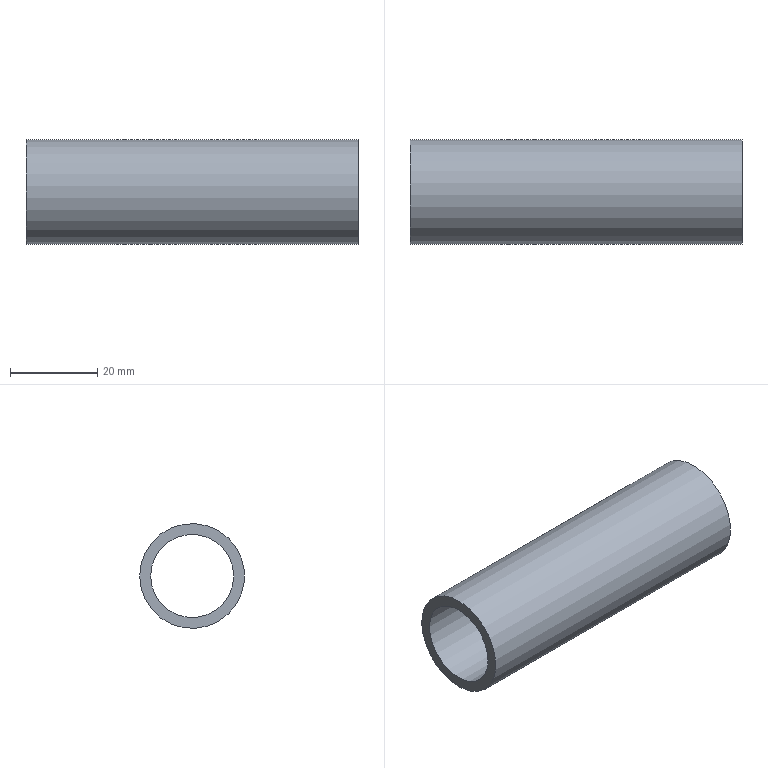Part | STEP file | 1-46.2 | 1 solid | 4 faces | box 76 x 24 x 24 mm | volume 12833 mm3 | plane 2 | cylinder 2 | commonest cylinder face diameters 19 x1 24 x1
STEP:
#1=CARTESIAN_POINT('',(0.,0.,0.));
#2=DIRECTION('',(0.,0.,1.));
#3=DIRECTION('',(1.,0.,0.));
#4=AXIS2_PLACEMENT_3D('',#1,#2,#3);
#5=CARTESIAN_POINT('',(38.,12.,0.));
#6=VERTEX_POINT('',#5);
#7=CARTESIAN_POINT('',(38.,0.,0.));
#8=DIRECTION('',(1.,0.,0.));
#9=DIRECTION('',(0.,1.,0.));
#10=AXIS2_PLACEMENT_3D('',#7,#8,#9);
#11=CIRCLE('',#10,12.);
#12=CARTESIAN_POINT('',(38.,-3.215,0.));
#13=DIRECTION('',(1.,0.,0.));
#14=DIRECTION('',(0.,1.,0.));
#15=AXIS2_PLACEMENT_3D('',#12,#13,#14);
#16=PLANE('',#15);
#17=CARTESIAN_POINT('',(3.215,0.));
#18=DIRECTION('',(1.,0.));
#19=AXIS2_PLACEMENT_2D('',#17,#18);
#20=CIRCLE('',#19,12.);
#21=(GEOMETRIC_REPRESENTATION_CONTEXT(2)PARAMETRIC_REPRESENTATION_CONTEXT()REPRESENTATION_CONTEXT('',''));
#22=DEFINITIONAL_REPRESENTATION('',(#20),#21);
#23=PCURVE('',#16,#22);
#24=CARTESIAN_POINT('',(38.,0.,0.));
#25=DIRECTION('',(-1.,0.,0.));
#26=DIRECTION('',(0.,1.,0.));
#27=AXIS2_PLACEMENT_3D('',#24,#25,#26);
#28=CYLINDRICAL_SURFACE('',#27,12.);
#29=CARTESIAN_POINT('',(6.283,0.));
#30=DIRECTION('',(-1.,0.));
#31=VECTOR('',#30,1.);
#32=LINE('',#29,#31);
#33=(GEOMETRIC_REPRESENTATION_CONTEXT(2)PARAMETRIC_REPRESENTATION_CONTEXT()REPRESENTATION_CONTEXT('',''));
#34=DEFINITIONAL_REPRESENTATION('',(#32),#33);
#35=PCURVE('',#28,#34);
#36=SURFACE_CURVE('',#11,(#23,#35),.PCURVE_S1.);
#37=EDGE_CURVE('',#6,#6,#36,.T.);
#38=ORIENTED_EDGE('',*,*,#37,.T.);
#39=EDGE_LOOP('',(#38));
#40=FACE_BOUND('',#39,.T.);
#41=CARTESIAN_POINT('',(38.,9.5,0.));
#42=VERTEX_POINT('',#41);
#43=CARTESIAN_POINT('',(38.,0.,0.));
#44=DIRECTION('',(-1.,0.,0.));
#45=DIRECTION('',(0.,1.,0.));
#46=AXIS2_PLACEMENT_3D('',#43,#44,#45);
#47=CIRCLE('',#46,9.5);
#48=CARTESIAN_POINT('',(12.715,0.));
#49=CARTESIAN_POINT('',(12.715,-16.454));
#50=CARTESIAN_POINT('',(-1.535,-8.227));
#51=CARTESIAN_POINT('',(-15.785,0.));
#52=CARTESIAN_POINT('',(-1.535,8.227));
#53=CARTESIAN_POINT('',(12.715,16.454));
#54=CARTESIAN_POINT('',(12.715,0.));
#55=(BOUNDED_CURVE()B_SPLINE_CURVE(2,(#48,#49,#50,#51,#52,#53,#54),.UNSPECIFIED.,.T.,.F.)B_SPLINE_CURVE_WITH_KNOTS((1,2,2,2,2,1),(-2.094,0.,2.094,4.189,6.283,8.378),.UNSPECIFIED.)CURVE()GEOMETRIC_REPRESENTATION_ITEM()RATIONAL_B_SPLINE_CURVE((1.,0.5,1.,0.5,1.,0.5,1.))REPRESENTATION_ITEM(''));
#56=(GEOMETRIC_REPRESENTATION_CONTEXT(2)PARAMETRIC_REPRESENTATION_CONTEXT()REPRESENTATION_CONTEXT('',''));
#57=DEFINITIONAL_REPRESENTATION('',(#55),#56);
#58=PCURVE('',#16,#57);
#59=CARTESIAN_POINT('',(38.,0.,0.));
#60=DIRECTION('',(-1.,0.,0.));
#61=DIRECTION('',(0.,1.,0.));
#62=AXIS2_PLACEMENT_3D('',#59,#60,#61);
#63=CYLINDRICAL_SURFACE('',#62,9.5);
#64=CARTESIAN_POINT('',(0.,0.));
#65=DIRECTION('',(1.,0.));
#66=VECTOR('',#65,1.);
#67=LINE('',#64,#66);
#68=(GEOMETRIC_REPRESENTATION_CONTEXT(2)PARAMETRIC_REPRESENTATION_CONTEXT()REPRESENTATION_CONTEXT('',''));
#69=DEFINITIONAL_REPRESENTATION('',(#67),#68);
#70=PCURVE('',#63,#69);
#71=SURFACE_CURVE('',#47,(#58,#70),.PCURVE_S1.);
#72=EDGE_CURVE('',#42,#42,#71,.T.);
#73=ORIENTED_EDGE('',*,*,#72,.T.);
#74=EDGE_LOOP('',(#73));
#75=FACE_BOUND('',#74,.T.);
#76=ADVANCED_FACE('',(#40,#75),#16,.T.);
#77=CARTESIAN_POINT('',(-38.,12.,0.));
#78=VERTEX_POINT('',#77);
#79=CARTESIAN_POINT('',(-38.,0.,0.));
#80=DIRECTION('',(1.,0.,0.));
#81=DIRECTION('',(0.,1.,0.));
#82=AXIS2_PLACEMENT_3D('',#79,#80,#81);
#83=CIRCLE('',#82,12.);
#84=CARTESIAN_POINT('',(-38.,-3.215,0.));
#85=DIRECTION('',(1.,0.,0.));
#86=DIRECTION('',(0.,1.,0.));
#87=AXIS2_PLACEMENT_3D('',#84,#85,#86);
#88=PLANE('',#87);
#89=CARTESIAN_POINT('',(3.215,0.));
#90=DIRECTION('',(1.,0.));
#91=AXIS2_PLACEMENT_2D('',#89,#90);
#92=CIRCLE('',#91,12.);
#93=(GEOMETRIC_REPRESENTATION_CONTEXT(2)PARAMETRIC_REPRESENTATION_CONTEXT()REPRESENTATION_CONTEXT('',''));
#94=DEFINITIONAL_REPRESENTATION('',(#92),#93);
#95=PCURVE('',#88,#94);
#96=CARTESIAN_POINT('',(6.283,76.));
#97=DIRECTION('',(-1.,0.));
#98=VECTOR('',#97,1.);
#99=LINE('',#96,#98);
#100=(GEOMETRIC_REPRESENTATION_CONTEXT(2)PARAMETRIC_REPRESENTATION_CONTEXT()REPRESENTATION_CONTEXT('',''));
#101=DEFINITIONAL_REPRESENTATION('',(#99),#100);
#102=PCURVE('',#28,#101);
#103=SURFACE_CURVE('',#83,(#95,#102),.PCURVE_S1.);
#104=EDGE_CURVE('',#78,#78,#103,.T.);
#105=ORIENTED_EDGE('',*,*,#104,.T.);
#106=EDGE_LOOP('',(#105));
#107=FACE_BOUND('',#106,.F.);
#108=CARTESIAN_POINT('',(-38.,9.5,0.));
#109=VERTEX_POINT('',#108);
#110=CARTESIAN_POINT('',(-38.,0.,0.));
#111=DIRECTION('',(-1.,0.,0.));
#112=DIRECTION('',(0.,1.,0.));
#113=AXIS2_PLACEMENT_3D('',#110,#111,#112);
#114=CIRCLE('',#113,9.5);
#115=CARTESIAN_POINT('',(12.715,0.));
#116=CARTESIAN_POINT('',(12.715,-16.454));
#117=CARTESIAN_POINT('',(-1.535,-8.227));
#118=CARTESIAN_POINT('',(-15.785,0.));
#119=CARTESIAN_POINT('',(-1.535,8.227));
#120=CARTESIAN_POINT('',(12.715,16.454));
#121=CARTESIAN_POINT('',(12.715,0.));
#122=(BOUNDED_CURVE()B_SPLINE_CURVE(2,(#115,#116,#117,#118,#119,#120,#121),.UNSPECIFIED.,.T.,.F.)B_SPLINE_CURVE_WITH_KNOTS((1,2,2,2,2,1),(-2.094,0.,2.094,4.189,6.283,8.378),.UNSPECIFIED.)CURVE()GEOMETRIC_REPRESENTATION_ITEM()RATIONAL_B_SPLINE_CURVE((1.,0.5,1.,0.5,1.,0.5,1.))REPRESENTATION_ITEM(''));
#123=(GEOMETRIC_REPRESENTATION_CONTEXT(2)PARAMETRIC_REPRESENTATION_CONTEXT()REPRESENTATION_CONTEXT('',''));
#124=DEFINITIONAL_REPRESENTATION('',(#122),#123);
#125=PCURVE('',#88,#124);
#126=CARTESIAN_POINT('',(0.,76.));
#127=DIRECTION('',(1.,0.));
#128=VECTOR('',#127,1.);
#129=LINE('',#126,#128);
#130=(GEOMETRIC_REPRESENTATION_CONTEXT(2)PARAMETRIC_REPRESENTATION_CONTEXT()REPRESENTATION_CONTEXT('',''));
#131=DEFINITIONAL_REPRESENTATION('',(#129),#130);
#132=PCURVE('',#63,#131);
#133=SURFACE_CURVE('',#114,(#125,#132),.PCURVE_S1.);
#134=EDGE_CURVE('',#109,#109,#133,.T.);
#135=ORIENTED_EDGE('',*,*,#134,.T.);
#136=EDGE_LOOP('',(#135));
#137=FACE_BOUND('',#136,.F.);
#138=ADVANCED_FACE('',(#107,#137),#88,.F.);
#139=CARTESIAN_POINT('',(38.,12.,0.));
#140=DIRECTION('',(-1.,0.,0.));
#141=VECTOR('',#140,1.);
#142=LINE('',#139,#141);
#143=CARTESIAN_POINT('',(6.283,0.));
#144=DIRECTION('',(0.,1.));
#145=VECTOR('',#144,1.);
#146=LINE('',#143,#145);
#147=(GEOMETRIC_REPRESENTATION_CONTEXT(2)PARAMETRIC_REPRESENTATION_CONTEXT()REPRESENTATION_CONTEXT('',''));
#148=DEFINITIONAL_REPRESENTATION('',(#146),#147);
#149=PCURVE('',#28,#148);
#150=CARTESIAN_POINT('',(0.,0.));
#151=DIRECTION('',(0.,1.));
#152=VECTOR('',#151,1.);
#153=LINE('',#150,#152);
#154=(GEOMETRIC_REPRESENTATION_CONTEXT(2)PARAMETRIC_REPRESENTATION_CONTEXT()REPRESENTATION_CONTEXT('',''));
#155=DEFINITIONAL_REPRESENTATION('',(#153),#154);
#156=PCURVE('',#28,#155);
#157=SEAM_CURVE('',#142,(#149,#156),.PCURVE_S1.);
#158=EDGE_CURVE('',#6,#78,#157,.T.);
#159=ORIENTED_EDGE('',*,*,#158,.T.);
#160=ORIENTED_EDGE('',*,*,#104,.T.);
#161=ORIENTED_EDGE('',*,*,#158,.F.);
#162=ORIENTED_EDGE('',*,*,#37,.F.);
#163=EDGE_LOOP('',(#159,#160,#161,#162));
#164=FACE_BOUND('',#163,.T.);
#165=ADVANCED_FACE('',(#164),#28,.T.);
#166=ORIENTED_EDGE('',*,*,#72,.T.);
#167=CARTESIAN_POINT('',(38.,9.5,0.));
#168=DIRECTION('',(-1.,0.,0.));
#169=VECTOR('',#168,1.);
#170=LINE('',#167,#169);
#171=CARTESIAN_POINT('',(6.283,0.));
#172=DIRECTION('',(0.,1.));
#173=VECTOR('',#172,1.);
#174=LINE('',#171,#173);
#175=(GEOMETRIC_REPRESENTATION_CONTEXT(2)PARAMETRIC_REPRESENTATION_CONTEXT()REPRESENTATION_CONTEXT('',''));
#176=DEFINITIONAL_REPRESENTATION('',(#174),#175);
#177=PCURVE('',#63,#176);
#178=CARTESIAN_POINT('',(0.,0.));
#179=DIRECTION('',(0.,1.));
#180=VECTOR('',#179,1.);
#181=LINE('',#178,#180);
#182=(GEOMETRIC_REPRESENTATION_CONTEXT(2)PARAMETRIC_REPRESENTATION_CONTEXT()REPRESENTATION_CONTEXT('',''));
#183=DEFINITIONAL_REPRESENTATION('',(#181),#182);
#184=PCURVE('',#63,#183);
#185=SEAM_CURVE('',#170,(#177,#184),.PCURVE_S1.);
#186=EDGE_CURVE('',#42,#109,#185,.T.);
#187=ORIENTED_EDGE('',*,*,#186,.T.);
#188=ORIENTED_EDGE('',*,*,#134,.F.);
#189=ORIENTED_EDGE('',*,*,#186,.F.);
#190=EDGE_LOOP('',(#166,#187,#188,#189));
#191=FACE_BOUND('',#190,.F.);
#192=ADVANCED_FACE('',(#191),#63,.F.);
#193=CLOSED_SHELL('',(#76,#138,#165,#192));
#194=MANIFOLD_SOLID_BREP('',#193);
#195=(LENGTH_UNIT()NAMED_UNIT(*)SI_UNIT(.MILLI.,.METRE.));
#196=UNCERTAINTY_MEASURE_WITH_UNIT(LENGTH_MEASURE(0.0000001),#195,'','');
#197=(NAMED_UNIT(*)PLANE_ANGLE_UNIT()SI_UNIT($,.RADIAN.));
#198=(NAMED_UNIT(*)SI_UNIT($,.STERADIAN.)SOLID_ANGLE_UNIT());
#199=(GEOMETRIC_REPRESENTATION_CONTEXT(3)GLOBAL_UNCERTAINTY_ASSIGNED_CONTEXT((#196))GLOBAL_UNIT_ASSIGNED_CONTEXT((#195,#197,#198))REPRESENTATION_CONTEXT('',''));
#200=ADVANCED_BREP_SHAPE_REPRESENTATION('',(#4,#194),#199);